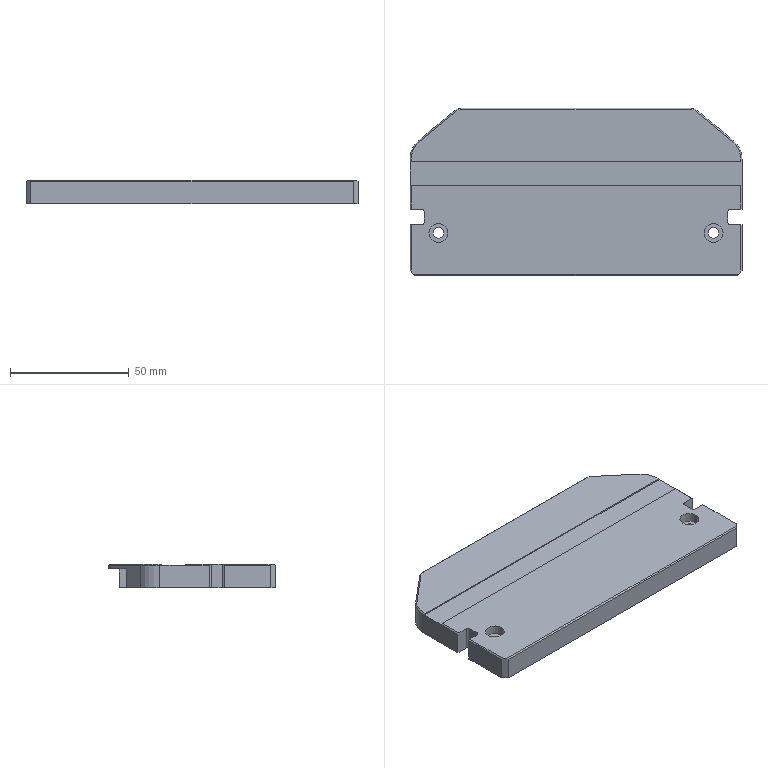Part | STEP file | SM140A-20-1140D-140A-600 Rear end plate | 1 solid | 74 faces | box 140 x 70.5 x 10 mm | volume 88188 mm3 | plane 46 | cylinder 24 | cone 4 | commonest cylinder face diameters 8 x6 2 x4 2.2 x4 4 x4 4.5 x4 20 x2